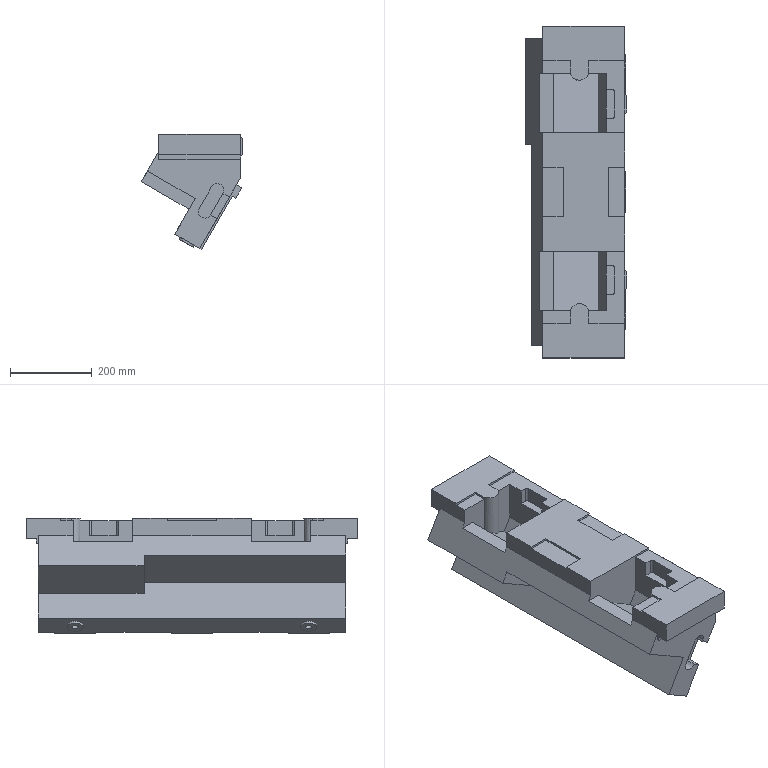Part | NX | features solid 2 | 1 solid | 152 faces | box 247.343 x 810 x 280.705 mm | volume 25045343 mm3 | plane 120 | cylinder 22 | cone 10 | commonest cylinder face diameters 10 x12 32 x4 16 x2 40 x2 45 x2